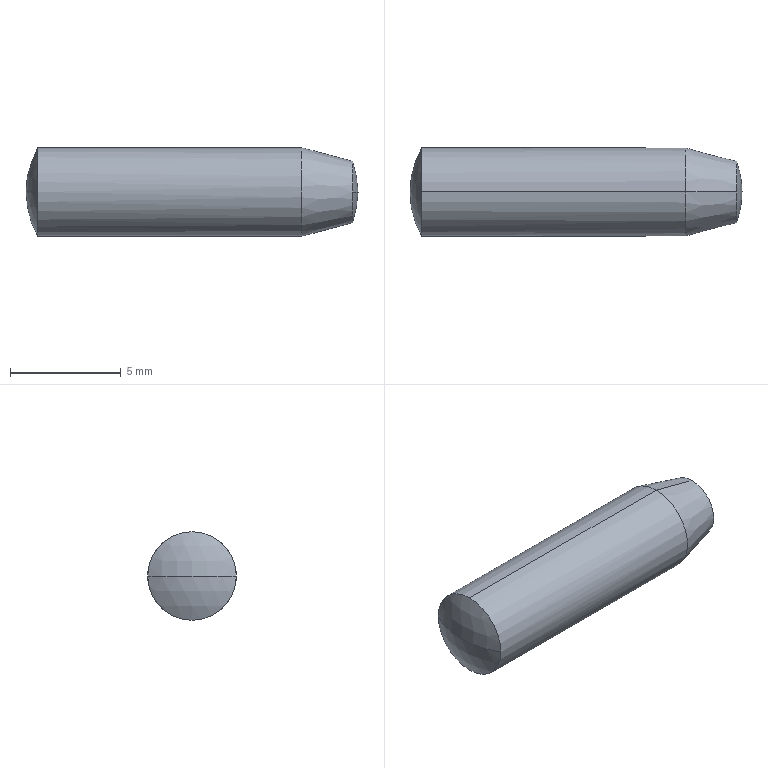Part | NX | features BREP 1 | 1 solid | 8 faces | box 15 x 4 x 4 mm | volume 174.937 mm3 | sphere 4 | cone 2 | cylinder 2 | commonest cylinder face diameters 4 x2
STEP:
#1=CARTESIAN_POINT('',(7.252,-1.387,0.));
#2=VERTEX_POINT('',#1);
#3=CARTESIAN_POINT('',(7.5,0.,0.));
#4=VERTEX_POINT('',#3);
#5=CARTESIAN_POINT('',(3.5,0.,0.));
#6=DIRECTION('',(0.,0.,-1.));
#7=DIRECTION('',(-1.,0.,0.));
#8=AXIS2_PLACEMENT_3D('',#5,#6,#7);
#9=CIRCLE('',#8,4.);
#10=EDGE_CURVE('',#2,#4,#9,.F.);
#11=ORIENTED_EDGE('',*,*,#10,.T.);
#12=CARTESIAN_POINT('',(7.252,1.387,0.));
#13=VERTEX_POINT('',#12);
#14=CARTESIAN_POINT('',(3.5,0.,0.));
#15=DIRECTION('',(0.,0.,1.));
#16=DIRECTION('',(0.,-1.,0.));
#17=AXIS2_PLACEMENT_3D('',#14,#15,#16);
#18=CIRCLE('',#17,4.);
#19=EDGE_CURVE('',#13,#4,#18,.F.);
#20=ORIENTED_EDGE('',*,*,#19,.F.);
#21=CARTESIAN_POINT('',(7.252,0.,1.387));
#22=VERTEX_POINT('',#21);
#23=CARTESIAN_POINT('',(7.252,0.,0.));
#24=DIRECTION('',(-1.,0.,0.));
#25=DIRECTION('',(0.,0.,1.));
#26=AXIS2_PLACEMENT_3D('',#23,#24,#25);
#27=CIRCLE('',#26,1.387);
#28=EDGE_CURVE('',#22,#13,#27,.T.);
#29=ORIENTED_EDGE('',*,*,#28,.F.);
#30=CARTESIAN_POINT('',(7.252,0.,0.));
#31=DIRECTION('',(-1.,0.,0.));
#32=DIRECTION('',(0.,0.,1.));
#33=AXIS2_PLACEMENT_3D('',#30,#31,#32);
#34=CIRCLE('',#33,1.387);
#35=EDGE_CURVE('',#2,#22,#34,.T.);
#36=ORIENTED_EDGE('',*,*,#35,.F.);
#37=EDGE_LOOP('',(#11,#20,#29,#36));
#38=FACE_BOUND('',#37,.T.);
#39=CARTESIAN_POINT('',(3.5,0.,0.));
#40=DIRECTION('',(0.,0.,1.));
#41=DIRECTION('',(0.,1.,0.));
#42=AXIS2_PLACEMENT_3D('',#39,#40,#41);
#43=SPHERICAL_SURFACE('',#42,4.);
#44=ADVANCED_FACE('',(#38),#43,.T.);
#45=ORIENTED_EDGE('',*,*,#28,.T.);
#46=CARTESIAN_POINT('',(7.252,0.,-1.387));
#47=VERTEX_POINT('',#46);
#48=CARTESIAN_POINT('',(7.252,0.,0.));
#49=DIRECTION('',(-1.,0.,0.));
#50=DIRECTION('',(0.,0.,1.));
#51=AXIS2_PLACEMENT_3D('',#48,#49,#50);
#52=CIRCLE('',#51,1.387);
#53=EDGE_CURVE('',#13,#47,#52,.T.);
#54=ORIENTED_EDGE('',*,*,#53,.T.);
#55=CARTESIAN_POINT('',(4.964,0.,-2.));
#56=VERTEX_POINT('',#55);
#57=CARTESIAN_POINT('',(7.252,0.,-1.387));
#58=DIRECTION('',(-0.9659,0.,-0.2588));
#59=VECTOR('',#58,1000.);
#60=LINE('',#57,#59);
#61=EDGE_CURVE('',#47,#56,#60,.T.);
#62=ORIENTED_EDGE('',*,*,#61,.T.);
#63=CARTESIAN_POINT('',(4.964,0.,2.));
#64=VERTEX_POINT('',#63);
#65=CARTESIAN_POINT('',(4.964,0.,0.));
#66=DIRECTION('',(-1.,0.,0.));
#67=DIRECTION('',(0.,0.,1.));
#68=AXIS2_PLACEMENT_3D('',#65,#66,#67);
#69=CIRCLE('',#68,2.);
#70=EDGE_CURVE('',#64,#56,#69,.T.);
#71=ORIENTED_EDGE('',*,*,#70,.F.);
#72=CARTESIAN_POINT('',(7.252,0.,1.387));
#73=DIRECTION('',(-0.9659,0.,0.2588));
#74=VECTOR('',#73,1000.);
#75=LINE('',#72,#74);
#76=EDGE_CURVE('',#22,#64,#75,.T.);
#77=ORIENTED_EDGE('',*,*,#76,.F.);
#78=EDGE_LOOP('',(#45,#54,#62,#71,#77));
#79=FACE_BOUND('',#78,.T.);
#80=CARTESIAN_POINT('',(7.252,0.,0.));
#81=DIRECTION('',(-1.,0.,0.));
#82=DIRECTION('',(0.,0.,-1.));
#83=AXIS2_PLACEMENT_3D('',#80,#81,#82);
#84=CONICAL_SURFACE('',#83,1.387,0.2618);
#85=ADVANCED_FACE('',(#79),#84,.T.);
#86=ORIENTED_EDGE('',*,*,#70,.T.);
#87=CARTESIAN_POINT('',(-6.964,0.,-2.));
#88=VERTEX_POINT('',#87);
#89=CARTESIAN_POINT('',(7.5,0.,-2.));
#90=DIRECTION('',(-1.,0.,0.));
#91=VECTOR('',#90,1000.);
#92=LINE('',#89,#91);
#93=EDGE_CURVE('',#56,#88,#92,.T.);
#94=ORIENTED_EDGE('',*,*,#93,.T.);
#95=CARTESIAN_POINT('',(-6.964,2.,0.));
#96=VERTEX_POINT('',#95);
#97=CARTESIAN_POINT('',(-6.964,0.,0.));
#98=DIRECTION('',(-1.,0.,0.));
#99=DIRECTION('',(0.,0.,1.));
#100=AXIS2_PLACEMENT_3D('',#97,#98,#99);
#101=CIRCLE('',#100,2.);
#102=EDGE_CURVE('',#96,#88,#101,.T.);
#103=ORIENTED_EDGE('',*,*,#102,.F.);
#104=CARTESIAN_POINT('',(-6.964,0.,2.));
#105=VERTEX_POINT('',#104);
#106=CARTESIAN_POINT('',(-6.964,0.,0.));
#107=DIRECTION('',(-1.,0.,0.));
#108=DIRECTION('',(0.,0.,1.));
#109=AXIS2_PLACEMENT_3D('',#106,#107,#108);
#110=CIRCLE('',#109,2.);
#111=EDGE_CURVE('',#105,#96,#110,.T.);
#112=ORIENTED_EDGE('',*,*,#111,.F.);
#113=CARTESIAN_POINT('',(7.5,0.,2.));
#114=DIRECTION('',(-1.,0.,0.));
#115=VECTOR('',#114,1000.);
#116=LINE('',#113,#115);
#117=EDGE_CURVE('',#64,#105,#116,.T.);
#118=ORIENTED_EDGE('',*,*,#117,.F.);
#119=EDGE_LOOP('',(#86,#94,#103,#112,#118));
#120=FACE_BOUND('',#119,.T.);
#121=CARTESIAN_POINT('',(7.5,0.,0.));
#122=DIRECTION('',(-1.,0.,0.));
#123=DIRECTION('',(0.,0.,-1.));
#124=AXIS2_PLACEMENT_3D('',#121,#122,#123);
#125=CYLINDRICAL_SURFACE('',#124,2.);
#126=ADVANCED_FACE('',(#120),#125,.T.);
#127=ORIENTED_EDGE('',*,*,#102,.T.);
#128=CARTESIAN_POINT('',(-6.964,-2.,0.));
#129=VERTEX_POINT('',#128);
#130=CARTESIAN_POINT('',(-6.964,0.,0.));
#131=DIRECTION('',(-1.,0.,0.));
#132=DIRECTION('',(0.,0.,1.));
#133=AXIS2_PLACEMENT_3D('',#130,#131,#132);
#134=CIRCLE('',#133,2.);
#135=EDGE_CURVE('',#88,#129,#134,.T.);
#136=ORIENTED_EDGE('',*,*,#135,.T.);
#137=CARTESIAN_POINT('',(-7.5,0.,0.));
#138=VERTEX_POINT('',#137);
#139=CARTESIAN_POINT('',(-3.5,0.,0.));
#140=DIRECTION('',(0.,0.,-1.));
#141=DIRECTION('',(0.,1.,0.));
#142=AXIS2_PLACEMENT_3D('',#139,#140,#141);
#143=CIRCLE('',#142,4.);
#144=EDGE_CURVE('',#129,#138,#143,.T.);
#145=ORIENTED_EDGE('',*,*,#144,.T.);
#146=CARTESIAN_POINT('',(-3.5,0.,0.));
#147=DIRECTION('',(0.,0.,1.));
#148=DIRECTION('',(1.,0.,0.));
#149=AXIS2_PLACEMENT_3D('',#146,#147,#148);
#150=CIRCLE('',#149,4.);
#151=EDGE_CURVE('',#96,#138,#150,.T.);
#152=ORIENTED_EDGE('',*,*,#151,.F.);
#153=EDGE_LOOP('',(#127,#136,#145,#152));
#154=FACE_BOUND('',#153,.T.);
#155=CARTESIAN_POINT('',(-3.5,0.,0.));
#156=DIRECTION('',(0.,0.,-1.));
#157=DIRECTION('',(0.,-1.,0.));
#158=AXIS2_PLACEMENT_3D('',#155,#156,#157);
#159=SPHERICAL_SURFACE('',#158,4.);
#160=ADVANCED_FACE('',(#154),#159,.T.);
#161=ORIENTED_EDGE('',*,*,#144,.F.);
#162=CARTESIAN_POINT('',(-6.964,0.,0.));
#163=DIRECTION('',(-1.,0.,0.));
#164=DIRECTION('',(0.,0.,1.));
#165=AXIS2_PLACEMENT_3D('',#162,#163,#164);
#166=CIRCLE('',#165,2.);
#167=EDGE_CURVE('',#129,#105,#166,.T.);
#168=ORIENTED_EDGE('',*,*,#167,.T.);
#169=ORIENTED_EDGE('',*,*,#111,.T.);
#170=ORIENTED_EDGE('',*,*,#151,.T.);
#171=EDGE_LOOP('',(#161,#168,#169,#170));
#172=FACE_BOUND('',#171,.T.);
#173=CARTESIAN_POINT('',(-3.5,0.,0.));
#174=DIRECTION('',(0.,0.,-1.));
#175=DIRECTION('',(0.,-1.,0.));
#176=AXIS2_PLACEMENT_3D('',#173,#174,#175);
#177=SPHERICAL_SURFACE('',#176,4.);
#178=ADVANCED_FACE('',(#172),#177,.T.);
#179=ORIENTED_EDGE('',*,*,#93,.F.);
#180=CARTESIAN_POINT('',(4.964,0.,0.));
#181=DIRECTION('',(-1.,0.,0.));
#182=DIRECTION('',(0.,0.,1.));
#183=AXIS2_PLACEMENT_3D('',#180,#181,#182);
#184=CIRCLE('',#183,2.);
#185=EDGE_CURVE('',#56,#64,#184,.T.);
#186=ORIENTED_EDGE('',*,*,#185,.T.);
#187=ORIENTED_EDGE('',*,*,#117,.T.);
#188=ORIENTED_EDGE('',*,*,#167,.F.);
#189=ORIENTED_EDGE('',*,*,#135,.F.);
#190=EDGE_LOOP('',(#179,#186,#187,#188,#189));
#191=FACE_BOUND('',#190,.T.);
#192=CARTESIAN_POINT('',(7.5,0.,0.));
#193=DIRECTION('',(-1.,0.,0.));
#194=DIRECTION('',(0.,0.,-1.));
#195=AXIS2_PLACEMENT_3D('',#192,#193,#194);
#196=CYLINDRICAL_SURFACE('',#195,2.);
#197=ADVANCED_FACE('',(#191),#196,.T.);
#198=ORIENTED_EDGE('',*,*,#61,.F.);
#199=CARTESIAN_POINT('',(7.252,0.,0.));
#200=DIRECTION('',(-1.,0.,0.));
#201=DIRECTION('',(0.,0.,1.));
#202=AXIS2_PLACEMENT_3D('',#199,#200,#201);
#203=CIRCLE('',#202,1.387);
#204=EDGE_CURVE('',#47,#2,#203,.T.);
#205=ORIENTED_EDGE('',*,*,#204,.T.);
#206=ORIENTED_EDGE('',*,*,#35,.T.);
#207=ORIENTED_EDGE('',*,*,#76,.T.);
#208=ORIENTED_EDGE('',*,*,#185,.F.);
#209=EDGE_LOOP('',(#198,#205,#206,#207,#208));
#210=FACE_BOUND('',#209,.T.);
#211=CARTESIAN_POINT('',(7.252,0.,0.));
#212=DIRECTION('',(-1.,0.,0.));
#213=DIRECTION('',(0.,0.,-1.));
#214=AXIS2_PLACEMENT_3D('',#211,#212,#213);
#215=CONICAL_SURFACE('',#214,1.387,0.2618);
#216=ADVANCED_FACE('',(#210),#215,.T.);
#217=ORIENTED_EDGE('',*,*,#19,.T.);
#218=ORIENTED_EDGE('',*,*,#10,.F.);
#219=ORIENTED_EDGE('',*,*,#204,.F.);
#220=ORIENTED_EDGE('',*,*,#53,.F.);
#221=EDGE_LOOP('',(#217,#218,#219,#220));
#222=FACE_BOUND('',#221,.T.);
#223=CARTESIAN_POINT('',(3.5,0.,0.));
#224=DIRECTION('',(0.,0.,1.));
#225=DIRECTION('',(0.,1.,0.));
#226=AXIS2_PLACEMENT_3D('',#223,#224,#225);
#227=SPHERICAL_SURFACE('',#226,4.);
#228=ADVANCED_FACE('',(#222),#227,.T.);
#229=CLOSED_SHELL('',(#44,#85,#126,#160,#178,#197,#216,#228));
#230=MANIFOLD_SOLID_BREP('',#229);
#231=(LENGTH_UNIT()NAMED_UNIT(*)SI_UNIT(.MILLI.,.METRE.));
#232=UNCERTAINTY_MEASURE_WITH_UNIT(LENGTH_MEASURE(0.00001),#231,'','');
#233=(NAMED_UNIT(*)PLANE_ANGLE_UNIT()SI_UNIT($,.RADIAN.));
#234=(NAMED_UNIT(*)SI_UNIT($,.STERADIAN.)SOLID_ANGLE_UNIT());
#235=(GEOMETRIC_REPRESENTATION_CONTEXT(3)GLOBAL_UNCERTAINTY_ASSIGNED_CONTEXT((#232))GLOBAL_UNIT_ASSIGNED_CONTEXT((#231,#233,#234))REPRESENTATION_CONTEXT('',''));
#236=ADVANCED_BREP_SHAPE_REPRESENTATION('',(#230),#235);